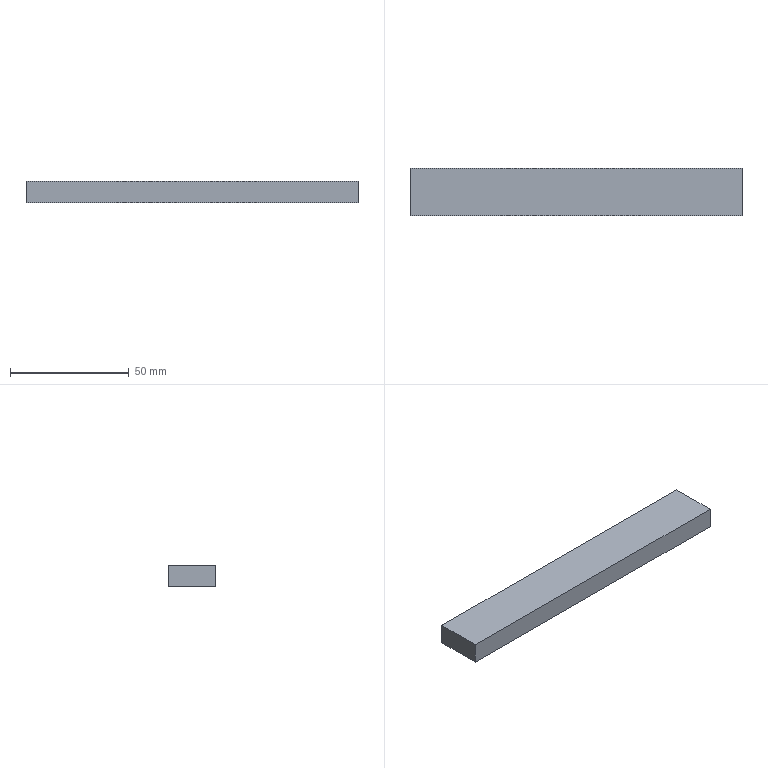Part | SolidWorks | features Extrusion 1 | 1 solid | 6 faces | box 140 x 20 x 9 mm | volume 25200 mm3 | plane 6
STEP:
#1=CARTESIAN_POINT('',(70.,-10.,0.));
#2=VERTEX_POINT('',#1);
#3=CARTESIAN_POINT('',(70.,10.,0.));
#4=VERTEX_POINT('',#3);
#5=CARTESIAN_POINT('',(70.,-10.,0.));
#6=DIRECTION('',(0.,1.,0.));
#7=VECTOR('',#6,1000.);
#8=LINE('',#5,#7);
#9=EDGE_CURVE('',#2,#4,#8,.T.);
#10=ORIENTED_EDGE('',*,*,#9,.T.);
#11=CARTESIAN_POINT('',(70.,10.,9.));
#12=VERTEX_POINT('',#11);
#13=CARTESIAN_POINT('',(70.,10.,9.));
#14=DIRECTION('',(0.,0.,-1.));
#15=VECTOR('',#14,1000.);
#16=LINE('',#13,#15);
#17=EDGE_CURVE('',#12,#4,#16,.T.);
#18=ORIENTED_EDGE('',*,*,#17,.F.);
#19=CARTESIAN_POINT('',(70.,-10.,9.));
#20=VERTEX_POINT('',#19);
#21=CARTESIAN_POINT('',(70.,-10.,9.));
#22=DIRECTION('',(0.,1.,0.));
#23=VECTOR('',#22,1000.);
#24=LINE('',#21,#23);
#25=EDGE_CURVE('',#20,#12,#24,.T.);
#26=ORIENTED_EDGE('',*,*,#25,.F.);
#27=CARTESIAN_POINT('',(70.,-10.,9.));
#28=DIRECTION('',(0.,0.,-1.));
#29=VECTOR('',#28,1000.);
#30=LINE('',#27,#29);
#31=EDGE_CURVE('',#20,#2,#30,.T.);
#32=ORIENTED_EDGE('',*,*,#31,.T.);
#33=EDGE_LOOP('',(#10,#18,#26,#32));
#34=FACE_OUTER_BOUND('',#33,.T.);
#35=CARTESIAN_POINT('',(70.,-10.,9.));
#36=DIRECTION('',(-1.,0.,0.));
#37=DIRECTION('',(0.,0.,1.));
#38=AXIS2_PLACEMENT_3D('',#35,#36,#37);
#39=PLANE('',#38);
#40=ADVANCED_FACE('',(#34),#39,.F.);
#41=CARTESIAN_POINT('',(-70.,10.,0.));
#42=VERTEX_POINT('',#41);
#43=CARTESIAN_POINT('',(-70.,10.,0.));
#44=DIRECTION('',(-1.,0.,0.));
#45=VECTOR('',#44,1000.);
#46=LINE('',#43,#45);
#47=EDGE_CURVE('',#4,#42,#46,.T.);
#48=ORIENTED_EDGE('',*,*,#47,.T.);
#49=CARTESIAN_POINT('',(-70.,10.,9.));
#50=VERTEX_POINT('',#49);
#51=CARTESIAN_POINT('',(-70.,10.,9.));
#52=DIRECTION('',(0.,0.,-1.));
#53=VECTOR('',#52,1000.);
#54=LINE('',#51,#53);
#55=EDGE_CURVE('',#50,#42,#54,.T.);
#56=ORIENTED_EDGE('',*,*,#55,.F.);
#57=CARTESIAN_POINT('',(-70.,10.,9.));
#58=DIRECTION('',(-1.,0.,0.));
#59=VECTOR('',#58,1000.);
#60=LINE('',#57,#59);
#61=EDGE_CURVE('',#12,#50,#60,.T.);
#62=ORIENTED_EDGE('',*,*,#61,.F.);
#63=ORIENTED_EDGE('',*,*,#17,.T.);
#64=EDGE_LOOP('',(#48,#56,#62,#63));
#65=FACE_OUTER_BOUND('',#64,.T.);
#66=CARTESIAN_POINT('',(-70.,10.,9.));
#67=DIRECTION('',(0.,-1.,0.));
#68=DIRECTION('',(0.,0.,-1.));
#69=AXIS2_PLACEMENT_3D('',#66,#67,#68);
#70=PLANE('',#69);
#71=ADVANCED_FACE('',(#65),#70,.F.);
#72=CARTESIAN_POINT('',(-70.,-10.,0.));
#73=VERTEX_POINT('',#72);
#74=CARTESIAN_POINT('',(-70.,-10.,0.));
#75=DIRECTION('',(0.,-1.,0.));
#76=VECTOR('',#75,1000.);
#77=LINE('',#74,#76);
#78=EDGE_CURVE('',#42,#73,#77,.T.);
#79=ORIENTED_EDGE('',*,*,#78,.T.);
#80=CARTESIAN_POINT('',(-70.,-10.,9.));
#81=VERTEX_POINT('',#80);
#82=CARTESIAN_POINT('',(-70.,-10.,9.));
#83=DIRECTION('',(0.,0.,-1.));
#84=VECTOR('',#83,1000.);
#85=LINE('',#82,#84);
#86=EDGE_CURVE('',#81,#73,#85,.T.);
#87=ORIENTED_EDGE('',*,*,#86,.F.);
#88=CARTESIAN_POINT('',(-70.,-10.,9.));
#89=DIRECTION('',(0.,-1.,0.));
#90=VECTOR('',#89,1000.);
#91=LINE('',#88,#90);
#92=EDGE_CURVE('',#50,#81,#91,.T.);
#93=ORIENTED_EDGE('',*,*,#92,.F.);
#94=ORIENTED_EDGE('',*,*,#55,.T.);
#95=EDGE_LOOP('',(#79,#87,#93,#94));
#96=FACE_OUTER_BOUND('',#95,.T.);
#97=CARTESIAN_POINT('',(-70.,-10.,9.));
#98=DIRECTION('',(1.,0.,0.));
#99=DIRECTION('',(0.,0.,-1.));
#100=AXIS2_PLACEMENT_3D('',#97,#98,#99);
#101=PLANE('',#100);
#102=ADVANCED_FACE('',(#96),#101,.F.);
#103=CARTESIAN_POINT('',(-70.,-10.,0.));
#104=DIRECTION('',(1.,0.,0.));
#105=VECTOR('',#104,1000.);
#106=LINE('',#103,#105);
#107=EDGE_CURVE('',#73,#2,#106,.T.);
#108=ORIENTED_EDGE('',*,*,#107,.T.);
#109=ORIENTED_EDGE('',*,*,#31,.F.);
#110=CARTESIAN_POINT('',(-70.,-10.,9.));
#111=DIRECTION('',(1.,0.,0.));
#112=VECTOR('',#111,1000.);
#113=LINE('',#110,#112);
#114=EDGE_CURVE('',#81,#20,#113,.T.);
#115=ORIENTED_EDGE('',*,*,#114,.F.);
#116=ORIENTED_EDGE('',*,*,#86,.T.);
#117=EDGE_LOOP('',(#108,#109,#115,#116));
#118=FACE_OUTER_BOUND('',#117,.T.);
#119=CARTESIAN_POINT('',(-70.,-10.,9.));
#120=DIRECTION('',(0.,1.,0.));
#121=DIRECTION('',(0.,0.,1.));
#122=AXIS2_PLACEMENT_3D('',#119,#120,#121);
#123=PLANE('',#122);
#124=ADVANCED_FACE('',(#118),#123,.F.);
#125=ORIENTED_EDGE('',*,*,#25,.T.);
#126=ORIENTED_EDGE('',*,*,#61,.T.);
#127=ORIENTED_EDGE('',*,*,#92,.T.);
#128=ORIENTED_EDGE('',*,*,#114,.T.);
#129=EDGE_LOOP('',(#125,#126,#127,#128));
#130=FACE_OUTER_BOUND('',#129,.T.);
#131=CARTESIAN_POINT('',(0.,0.,9.));
#132=DIRECTION('',(0.,0.,-1.));
#133=DIRECTION('',(-1.,0.,0.));
#134=AXIS2_PLACEMENT_3D('',#131,#132,#133);
#135=PLANE('',#134);
#136=ADVANCED_FACE('',(#130),#135,.F.);
#137=ORIENTED_EDGE('',*,*,#9,.F.);
#138=ORIENTED_EDGE('',*,*,#107,.F.);
#139=ORIENTED_EDGE('',*,*,#78,.F.);
#140=ORIENTED_EDGE('',*,*,#47,.F.);
#141=EDGE_LOOP('',(#137,#138,#139,#140));
#142=FACE_OUTER_BOUND('',#141,.T.);
#143=CARTESIAN_POINT('',(0.,0.,0.));
#144=DIRECTION('',(0.,0.,-1.));
#145=DIRECTION('',(-1.,0.,0.));
#146=AXIS2_PLACEMENT_3D('',#143,#144,#145);
#147=PLANE('',#146);
#148=ADVANCED_FACE('',(#142),#147,.T.);
#149=CLOSED_SHELL('',(#40,#71,#102,#124,#136,#148));
#150=MANIFOLD_SOLID_BREP('',#149);
#151=CARTESIAN_POINT('',(0.,0.,0.));
#152=DIRECTION('',(0.,0.,1.));
#153=DIRECTION('',(1.,0.,0.));
#154=AXIS2_PLACEMENT_3D('',#151,#152,#153);
#155=(LENGTH_UNIT()NAMED_UNIT(*)SI_UNIT(.MILLI.,.METRE.));
#156=UNCERTAINTY_MEASURE_WITH_UNIT(LENGTH_MEASURE(0.00001),#155,'','');
#157=(NAMED_UNIT(*)PLANE_ANGLE_UNIT()SI_UNIT($,.RADIAN.));
#158=(NAMED_UNIT(*)SI_UNIT($,.STERADIAN.)SOLID_ANGLE_UNIT());
#159=(GEOMETRIC_REPRESENTATION_CONTEXT(3)GLOBAL_UNCERTAINTY_ASSIGNED_CONTEXT((#156))GLOBAL_UNIT_ASSIGNED_CONTEXT((#155,#157,#158))REPRESENTATION_CONTEXT('',''));
#160=ADVANCED_BREP_SHAPE_REPRESENTATION('',(#150,#154),#159);